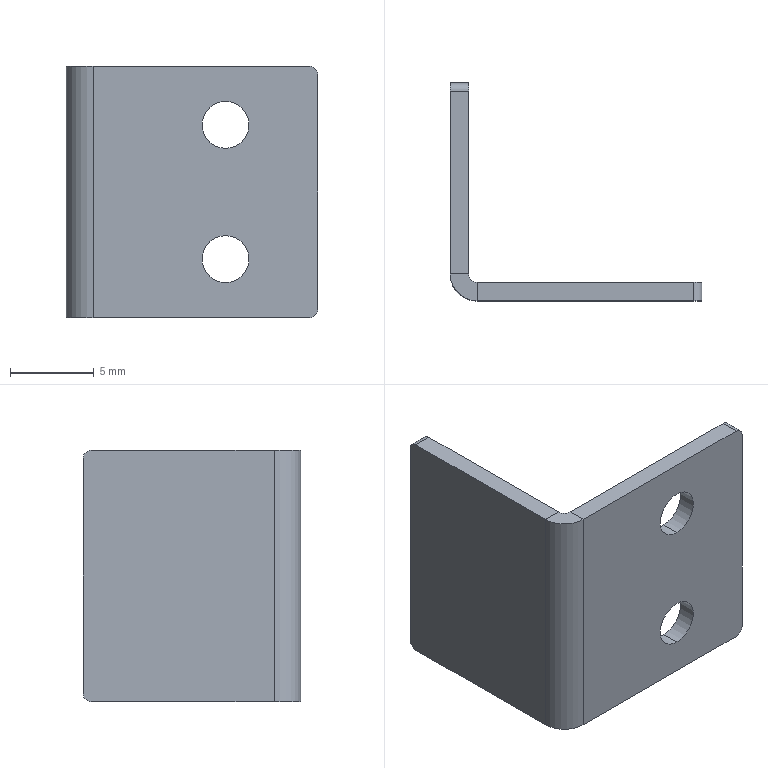Part | STEP file | Single-axis module KK photoelectric shield | 1 solid | 22 faces | box 15 x 13 x 15 mm | volume 422.631 mm3 | plane 12 | cylinder 10 | commonest cylinder face diameters 1 x5 2.8 x4 3.2 x1